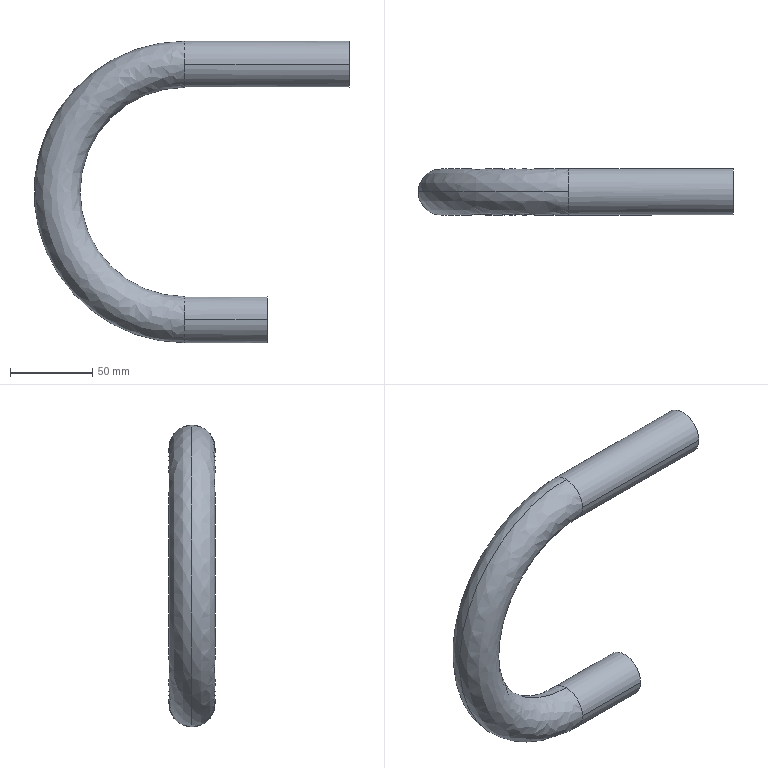Part | STEP file | copper tube 16_default_machined_ | 1 solid | 14 faces | box 191.58 x 28 x 183.16 mm | volume 49168 mm3 | cylinder 8 | spline 4 | plane 2 | commonest cylinder face diameters 25 x4 28 x4